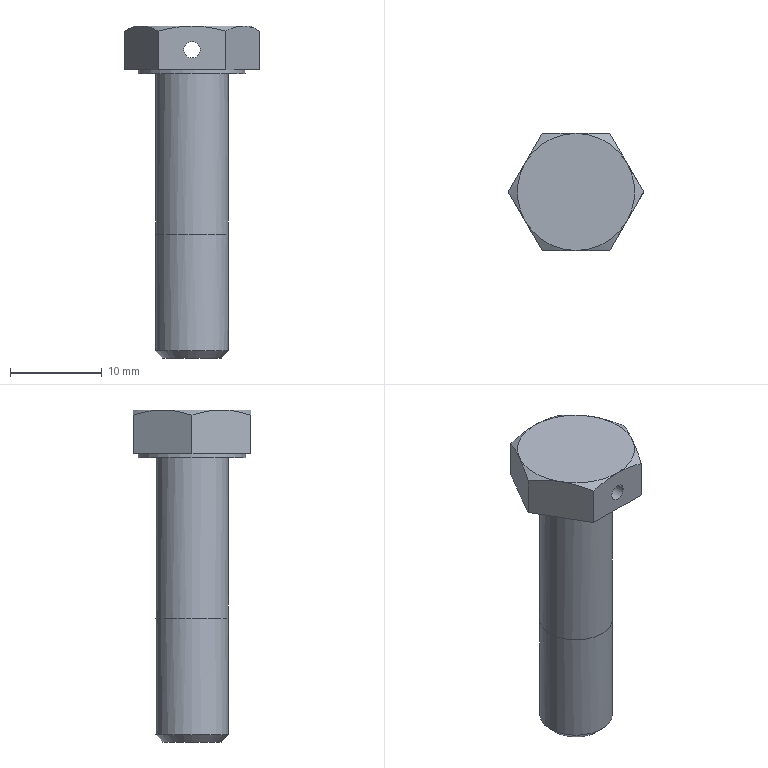Part | NX | features solid 2 | 1 solid | 21 faces | box 14.723 x 12.751 x 36.138 mm | volume 2207 mm3 | plane 10 | cone 7 | cylinder 4 | commonest cylinder face diameters 7.938 x2 1.778 x1 11.684 x1
STEP:
#1=CARTESIAN_POINT('',(-3.969,0.,-5.182));
#2=VERTEX_POINT('',#1);
#3=CARTESIAN_POINT('',(0.,0.,-5.182));
#4=DIRECTION('',(0.,0.,-1.));
#5=DIRECTION('',(-1.,0.,0.));
#6=AXIS2_PLACEMENT_3D('',#3,#4,#5);
#7=CIRCLE('',#6,3.969);
#8=EDGE_CURVE('',#2,#2,#7,.T.);
#9=ORIENTED_EDGE('',*,*,#8,.T.);
#10=EDGE_LOOP('',(#9));
#11=FACE_BOUND('',#10,.T.);
#12=CARTESIAN_POINT('',(-3.969,0.,-22.644));
#13=VERTEX_POINT('',#12);
#14=CARTESIAN_POINT('',(-3.11,3.11,-22.644));
#15=CARTESIAN_POINT('',(-4.398,0.,-22.644));
#16=CARTESIAN_POINT('',(-3.11,-3.11,-22.644));
#17=CARTESIAN_POINT('',(0.,-4.398,-22.644));
#18=CARTESIAN_POINT('',(3.11,-3.11,-22.644));
#19=CARTESIAN_POINT('',(4.398,0.,-22.644));
#20=CARTESIAN_POINT('',(3.11,3.11,-22.644));
#21=CARTESIAN_POINT('',(0.,4.398,-22.644));
#22=CARTESIAN_POINT('',(-3.11,3.11,-22.644));
#23=CARTESIAN_POINT('',(-4.398,0.,-22.644));
#24=CARTESIAN_POINT('',(-3.11,-3.11,-22.644));
#25=B_SPLINE_CURVE_WITH_KNOTS('',3,(#14,#15,#16,#17,#18,#19,#20,#21,#22,#23,#24),.UNSPECIFIED.,.T.,.F.,(1,1,1,1,1,1,1,1,1,1,1,1,1,1,1),(-0.375,-0.25,-0.125,0.,0.125,0.25,0.375,0.5,0.625,0.75,0.875,1.,1.125,1.25,1.375),.UNSPECIFIED.);
#26=EDGE_CURVE('',#13,#13,#25,.T.);
#27=ORIENTED_EDGE('',*,*,#26,.T.);
#28=EDGE_LOOP('',(#27));
#29=FACE_BOUND('',#28,.T.);
#30=CARTESIAN_POINT('',(0.,0.,0.));
#31=DIRECTION('',(0.,0.,-1.));
#32=DIRECTION('',(-1.,0.,0.));
#33=AXIS2_PLACEMENT_3D('',#30,#31,#32);
#34=CYLINDRICAL_SURFACE('',#33,3.969);
#35=ADVANCED_FACE('',(#11,#29),#34,.T.);
#36=CARTESIAN_POINT('',(-7.362,0.,-4.775));
#37=VERTEX_POINT('',#36);
#38=CARTESIAN_POINT('',(-3.681,6.375,-4.775));
#39=VERTEX_POINT('',#38);
#40=CARTESIAN_POINT('',(-4.061,5.717,-4.775));
#41=DIRECTION('',(0.5,0.866,0.));
#42=VECTOR('',#41,1000.);
#43=LINE('',#40,#42);
#44=EDGE_CURVE('',#37,#39,#43,.T.);
#45=ORIENTED_EDGE('',*,*,#44,.T.);
#46=CARTESIAN_POINT('',(3.681,6.375,-4.775));
#47=VERTEX_POINT('',#46);
#48=CARTESIAN_POINT('',(5.842,6.375,-4.775));
#49=DIRECTION('',(1.,0.,0.));
#50=VECTOR('',#49,1000.);
#51=LINE('',#48,#50);
#52=EDGE_CURVE('',#39,#47,#51,.T.);
#53=ORIENTED_EDGE('',*,*,#52,.T.);
#54=CARTESIAN_POINT('',(7.362,0.,-4.775));
#55=VERTEX_POINT('',#54);
#56=CARTESIAN_POINT('',(6.982,0.658,-4.775));
#57=DIRECTION('',(0.5,-0.866,0.));
#58=VECTOR('',#57,1000.);
#59=LINE('',#56,#58);
#60=EDGE_CURVE('',#47,#55,#59,.T.);
#61=ORIENTED_EDGE('',*,*,#60,.T.);
#62=CARTESIAN_POINT('',(3.681,-6.375,-4.775));
#63=VERTEX_POINT('',#62);
#64=CARTESIAN_POINT('',(6.982,-0.658,-4.775));
#65=DIRECTION('',(-0.5,-0.866,0.));
#66=VECTOR('',#65,1000.);
#67=LINE('',#64,#66);
#68=EDGE_CURVE('',#55,#63,#67,.T.);
#69=ORIENTED_EDGE('',*,*,#68,.T.);
#70=CARTESIAN_POINT('',(-3.681,-6.375,-4.775));
#71=VERTEX_POINT('',#70);
#72=CARTESIAN_POINT('',(5.842,-6.375,-4.775));
#73=DIRECTION('',(-1.,0.,0.));
#74=VECTOR('',#73,1000.);
#75=LINE('',#72,#74);
#76=EDGE_CURVE('',#63,#71,#75,.T.);
#77=ORIENTED_EDGE('',*,*,#76,.T.);
#78=CARTESIAN_POINT('',(-4.061,-5.717,-4.775));
#79=DIRECTION('',(-0.5,0.866,0.));
#80=VECTOR('',#79,1000.);
#81=LINE('',#78,#80);
#82=EDGE_CURVE('',#71,#37,#81,.T.);
#83=ORIENTED_EDGE('',*,*,#82,.T.);
#84=EDGE_LOOP('',(#45,#53,#61,#69,#77,#83));
#85=FACE_BOUND('',#84,.T.);
#86=CARTESIAN_POINT('',(-5.842,0.,-4.775));
#87=VERTEX_POINT('',#86);
#88=CARTESIAN_POINT('',(0.,0.,-4.775));
#89=DIRECTION('',(0.,0.,-1.));
#90=DIRECTION('',(-1.,0.,0.));
#91=AXIS2_PLACEMENT_3D('',#88,#89,#90);
#92=CIRCLE('',#91,5.842);
#93=EDGE_CURVE('',#87,#87,#92,.T.);
#94=ORIENTED_EDGE('',*,*,#93,.F.);
#95=EDGE_LOOP('',(#94));
#96=FACE_BOUND('',#95,.T.);
#97=CARTESIAN_POINT('',(5.842,0.,-4.775));
#98=DIRECTION('',(0.,0.,-1.));
#99=DIRECTION('',(-1.,0.,0.));
#100=AXIS2_PLACEMENT_3D('',#97,#98,#99);
#101=PLANE('',#100);
#102=ADVANCED_FACE('',(#85,#96),#101,.T.);
#103=CARTESIAN_POINT('',(-3.181,0.,-36.138));
#104=VERTEX_POINT('',#103);
#105=CARTESIAN_POINT('',(0.,0.,-36.138));
#106=DIRECTION('',(0.,0.,-1.));
#107=DIRECTION('',(-1.,0.,0.));
#108=AXIS2_PLACEMENT_3D('',#105,#106,#107);
#109=CIRCLE('',#108,3.181);
#110=EDGE_CURVE('',#104,#104,#109,.T.);
#111=ORIENTED_EDGE('',*,*,#110,.T.);
#112=EDGE_LOOP('',(#111));
#113=FACE_BOUND('',#112,.T.);
#114=CARTESIAN_POINT('',(0.,0.,-36.138));
#115=DIRECTION('',(0.,0.,-1.));
#116=DIRECTION('',(-1.,0.,0.));
#117=AXIS2_PLACEMENT_3D('',#114,#115,#116);
#118=PLANE('',#117);
#119=ADVANCED_FACE('',(#113),#118,.T.);
#120=CARTESIAN_POINT('',(-3.969,0.,-35.35));
#121=VERTEX_POINT('',#120);
#122=CARTESIAN_POINT('',(0.,0.,-35.35));
#123=DIRECTION('',(0.,0.,-1.));
#124=DIRECTION('',(-1.,0.,0.));
#125=AXIS2_PLACEMENT_3D('',#122,#123,#124);
#126=CIRCLE('',#125,3.969);
#127=EDGE_CURVE('',#121,#121,#126,.T.);
#128=ORIENTED_EDGE('',*,*,#127,.T.);
#129=EDGE_LOOP('',(#128));
#130=FACE_BOUND('',#129,.T.);
#131=ORIENTED_EDGE('',*,*,#110,.F.);
#132=EDGE_LOOP('',(#131));
#133=FACE_BOUND('',#132,.T.);
#134=CARTESIAN_POINT('',(0.,0.,-36.138));
#135=DIRECTION('',(0.,0.,1.));
#136=DIRECTION('',(1.,0.,0.));
#137=AXIS2_PLACEMENT_3D('',#134,#135,#136);
#138=CONICAL_SURFACE('',#137,3.181,0.7854);
#139=ADVANCED_FACE('',(#130,#133),#138,.T.);
#140=ORIENTED_EDGE('',*,*,#26,.F.);
#141=EDGE_LOOP('',(#140));
#142=FACE_BOUND('',#141,.T.);
#143=ORIENTED_EDGE('',*,*,#127,.F.);
#144=EDGE_LOOP('',(#143));
#145=FACE_BOUND('',#144,.T.);
#146=CARTESIAN_POINT('',(0.,0.,0.));
#147=DIRECTION('',(0.,0.,-1.));
#148=DIRECTION('',(-1.,0.,0.));
#149=AXIS2_PLACEMENT_3D('',#146,#147,#148);
#150=CYLINDRICAL_SURFACE('',#149,3.969);
#151=ADVANCED_FACE('',(#142,#145),#150,.T.);
#152=CARTESIAN_POINT('',(-5.842,0.,-5.182));
#153=VERTEX_POINT('',#152);
#154=CARTESIAN_POINT('',(0.,0.,-5.182));
#155=DIRECTION('',(0.,0.,-1.));
#156=DIRECTION('',(-1.,0.,0.));
#157=AXIS2_PLACEMENT_3D('',#154,#155,#156);
#158=CIRCLE('',#157,5.842);
#159=EDGE_CURVE('',#153,#153,#158,.T.);
#160=ORIENTED_EDGE('',*,*,#159,.T.);
#161=EDGE_LOOP('',(#160));
#162=FACE_BOUND('',#161,.T.);
#163=ORIENTED_EDGE('',*,*,#8,.F.);
#164=EDGE_LOOP('',(#163));
#165=FACE_BOUND('',#164,.T.);
#166=CARTESIAN_POINT('',(3.969,0.,-5.182));
#167=DIRECTION('',(0.,0.,-1.));
#168=DIRECTION('',(-1.,0.,0.));
#169=AXIS2_PLACEMENT_3D('',#166,#167,#168);
#170=PLANE('',#169);
#171=ADVANCED_FACE('',(#162,#165),#170,.T.);
#172=ORIENTED_EDGE('',*,*,#93,.T.);
#173=EDGE_LOOP('',(#172));
#174=FACE_BOUND('',#173,.T.);
#175=ORIENTED_EDGE('',*,*,#159,.F.);
#176=EDGE_LOOP('',(#175));
#177=FACE_BOUND('',#176,.T.);
#178=CARTESIAN_POINT('',(0.,0.,0.));
#179=DIRECTION('',(0.,0.,-1.));
#180=DIRECTION('',(-1.,0.,0.));
#181=AXIS2_PLACEMENT_3D('',#178,#179,#180);
#182=CYLINDRICAL_SURFACE('',#181,5.842);
#183=ADVANCED_FACE('',(#174,#177),#182,.T.);
#184=CARTESIAN_POINT('',(0.,6.375,-1.702));
#185=VERTEX_POINT('',#184);
#186=CARTESIAN_POINT('',(0.,6.375,-2.591));
#187=DIRECTION('',(0.,1.,0.));
#188=DIRECTION('',(0.,0.,1.));
#189=AXIS2_PLACEMENT_3D('',#186,#187,#188);
#190=CIRCLE('',#189,0.889);
#191=EDGE_CURVE('',#185,#185,#190,.T.);
#192=ORIENTED_EDGE('',*,*,#191,.F.);
#193=EDGE_LOOP('',(#192));
#194=FACE_BOUND('',#193,.T.);
#195=ORIENTED_EDGE('',*,*,#52,.F.);
#196=CARTESIAN_POINT('',(-3.681,6.375,-0.5694));
#197=VERTEX_POINT('',#196);
#198=CARTESIAN_POINT('',(-3.681,6.375,-39.752));
#199=DIRECTION('',(0.,0.,1.));
#200=VECTOR('',#199,1000.);
#201=LINE('',#198,#200);
#202=EDGE_CURVE('',#39,#197,#201,.T.);
#203=ORIENTED_EDGE('',*,*,#202,.T.);
#204=CARTESIAN_POINT('',(0.,6.375,0.));
#205=VERTEX_POINT('',#204);
#206=CARTESIAN_POINT('',(-3.681,6.375,-0.5694));
#207=CARTESIAN_POINT('',(-2.484,6.375,-0.2238));
#208=CARTESIAN_POINT('',(-1.244,6.375,0.));
#209=CARTESIAN_POINT('',(0.,6.375,0.));
#210=B_SPLINE_CURVE_WITH_KNOTS('',3,(#206,#207,#208,#209),.UNSPECIFIED.,.F.,.F.,(4,4),(0.006567,0.01029),.UNSPECIFIED.);
#211=EDGE_CURVE('',#205,#197,#210,.F.);
#212=ORIENTED_EDGE('',*,*,#211,.F.);
#213=CARTESIAN_POINT('',(3.681,6.375,-0.5694));
#214=VERTEX_POINT('',#213);
#215=CARTESIAN_POINT('',(0.,6.375,0.));
#216=CARTESIAN_POINT('',(1.245,6.375,0.));
#217=CARTESIAN_POINT('',(2.49,6.375,-0.2258));
#218=CARTESIAN_POINT('',(3.681,6.375,-0.5694));
#219=B_SPLINE_CURVE_WITH_KNOTS('',3,(#215,#216,#217,#218),.UNSPECIFIED.,.F.,.F.,(4,4),(0.01029,0.01402),.UNSPECIFIED.);
#220=EDGE_CURVE('',#214,#205,#219,.F.);
#221=ORIENTED_EDGE('',*,*,#220,.F.);
#222=CARTESIAN_POINT('',(3.681,6.375,-39.752));
#223=DIRECTION('',(0.,0.,1.));
#224=VECTOR('',#223,1000.);
#225=LINE('',#222,#224);
#226=EDGE_CURVE('',#47,#214,#225,.T.);
#227=ORIENTED_EDGE('',*,*,#226,.F.);
#228=EDGE_LOOP('',(#195,#203,#212,#221,#227));
#229=FACE_BOUND('',#228,.T.);
#230=CARTESIAN_POINT('',(3.681,6.375,-39.752));
#231=DIRECTION('',(0.,1.,0.));
#232=DIRECTION('',(0.,0.,1.));
#233=AXIS2_PLACEMENT_3D('',#230,#231,#232);
#234=PLANE('',#233);
#235=ADVANCED_FACE('',(#194,#229),#234,.T.);
#236=ORIENTED_EDGE('',*,*,#44,.F.);
#237=CARTESIAN_POINT('',(-7.362,0.,-0.5694));
#238=VERTEX_POINT('',#237);
#239=CARTESIAN_POINT('',(-7.362,0.,-39.752));
#240=DIRECTION('',(0.,0.,1.));
#241=VECTOR('',#240,1000.);
#242=LINE('',#239,#241);
#243=EDGE_CURVE('',#37,#238,#242,.T.);
#244=ORIENTED_EDGE('',*,*,#243,.T.);
#245=CARTESIAN_POINT('',(-5.521,3.188,0.));
#246=VERTEX_POINT('',#245);
#247=CARTESIAN_POINT('',(-5.521,3.188,0.));
#248=CARTESIAN_POINT('',(-6.146,2.106,0.));
#249=CARTESIAN_POINT('',(-6.761,1.04,-0.2227));
#250=CARTESIAN_POINT('',(-7.362,0.,-0.5694));
#251=B_SPLINE_CURVE_WITH_KNOTS('',3,(#247,#248,#249,#250),.UNSPECIFIED.,.F.,.F.,(4,4),(0.003725,0.007435),.UNSPECIFIED.);
#252=EDGE_CURVE('',#246,#238,#251,.T.);
#253=ORIENTED_EDGE('',*,*,#252,.F.);
#254=CARTESIAN_POINT('',(-3.681,6.375,-0.5694));
#255=CARTESIAN_POINT('',(-4.283,5.332,-0.2218));
#256=CARTESIAN_POINT('',(-4.894,4.274,0.));
#257=CARTESIAN_POINT('',(-5.521,3.188,0.));
#258=B_SPLINE_CURVE_WITH_KNOTS('',3,(#254,#255,#256,#257),.UNSPECIFIED.,.F.,.F.,(4,4),(0.000000238,0.003725),.UNSPECIFIED.);
#259=EDGE_CURVE('',#197,#246,#258,.T.);
#260=ORIENTED_EDGE('',*,*,#259,.F.);
#261=ORIENTED_EDGE('',*,*,#202,.F.);
#262=EDGE_LOOP('',(#236,#244,#253,#260,#261));
#263=FACE_BOUND('',#262,.T.);
#264=CARTESIAN_POINT('',(-3.681,6.375,-39.752));
#265=DIRECTION('',(-0.866,0.5,0.));
#266=DIRECTION('',(-0.5,-0.866,0.));
#267=AXIS2_PLACEMENT_3D('',#264,#265,#266);
#268=PLANE('',#267);
#269=ADVANCED_FACE('',(#263),#268,.T.);
#270=ORIENTED_EDGE('',*,*,#82,.F.);
#271=CARTESIAN_POINT('',(-3.681,-6.375,-0.5694));
#272=VERTEX_POINT('',#271);
#273=CARTESIAN_POINT('',(-3.681,-6.375,-39.752));
#274=DIRECTION('',(0.,0.,1.));
#275=VECTOR('',#274,1000.);
#276=LINE('',#273,#275);
#277=EDGE_CURVE('',#71,#272,#276,.T.);
#278=ORIENTED_EDGE('',*,*,#277,.T.);
#279=CARTESIAN_POINT('',(-5.521,-3.188,0.));
#280=VERTEX_POINT('',#279);
#281=CARTESIAN_POINT('',(-5.521,-3.188,0.));
#282=CARTESIAN_POINT('',(-4.896,-4.27,0.));
#283=CARTESIAN_POINT('',(-4.281,-5.335,-0.2227));
#284=CARTESIAN_POINT('',(-3.681,-6.375,-0.5694));
#285=B_SPLINE_CURVE_WITH_KNOTS('',3,(#281,#282,#283,#284),.UNSPECIFIED.,.F.,.F.,(4,4),(0.003725,0.007435),.UNSPECIFIED.);
#286=EDGE_CURVE('',#280,#272,#285,.T.);
#287=ORIENTED_EDGE('',*,*,#286,.F.);
#288=CARTESIAN_POINT('',(-7.362,0.,-0.5694));
#289=CARTESIAN_POINT('',(-6.76,-1.043,-0.2218));
#290=CARTESIAN_POINT('',(-6.148,-2.102,0.));
#291=CARTESIAN_POINT('',(-5.521,-3.188,0.));
#292=B_SPLINE_CURVE_WITH_KNOTS('',3,(#288,#289,#290,#291),.UNSPECIFIED.,.F.,.F.,(4,4),(0.000000238,0.003725),.UNSPECIFIED.);
#293=EDGE_CURVE('',#238,#280,#292,.T.);
#294=ORIENTED_EDGE('',*,*,#293,.F.);
#295=ORIENTED_EDGE('',*,*,#243,.F.);
#296=EDGE_LOOP('',(#270,#278,#287,#294,#295));
#297=FACE_BOUND('',#296,.T.);
#298=CARTESIAN_POINT('',(-7.362,0.,-39.752));
#299=DIRECTION('',(-0.866,-0.5,0.));
#300=DIRECTION('',(0.5,-0.866,0.));
#301=AXIS2_PLACEMENT_3D('',#298,#299,#300);
#302=PLANE('',#301);
#303=ADVANCED_FACE('',(#297),#302,.T.);
#304=CARTESIAN_POINT('',(0.,-6.375,-3.48));
#305=VERTEX_POINT('',#304);
#306=CARTESIAN_POINT('',(0.,-6.375,-2.591));
#307=DIRECTION('',(0.,-1.,0.));
#308=DIRECTION('',(0.,0.,-1.));
#309=AXIS2_PLACEMENT_3D('',#306,#307,#308);
#310=CIRCLE('',#309,0.889);
#311=EDGE_CURVE('',#305,#305,#310,.T.);
#312=ORIENTED_EDGE('',*,*,#311,.F.);
#313=EDGE_LOOP('',(#312));
#314=FACE_BOUND('',#313,.T.);
#315=ORIENTED_EDGE('',*,*,#76,.F.);
#316=CARTESIAN_POINT('',(3.681,-6.375,-0.5694));
#317=VERTEX_POINT('',#316);
#318=CARTESIAN_POINT('',(3.681,-6.375,-39.752));
#319=DIRECTION('',(0.,0.,1.));
#320=VECTOR('',#319,1000.);
#321=LINE('',#318,#320);
#322=EDGE_CURVE('',#63,#317,#321,.T.);
#323=ORIENTED_EDGE('',*,*,#322,.T.);
#324=CARTESIAN_POINT('',(0.,-6.375,0.));
#325=VERTEX_POINT('',#324);
#326=CARTESIAN_POINT('',(0.,-6.375,0.));
#327=CARTESIAN_POINT('',(1.245,-6.375,0.));
#328=CARTESIAN_POINT('',(2.49,-6.375,-0.2258));
#329=CARTESIAN_POINT('',(3.681,-6.375,-0.5694));
#330=B_SPLINE_CURVE_WITH_KNOTS('',3,(#326,#327,#328,#329),.UNSPECIFIED.,.F.,.F.,(4,4),(0.01029,0.01402),.UNSPECIFIED.);
#331=EDGE_CURVE('',#325,#317,#330,.T.);
#332=ORIENTED_EDGE('',*,*,#331,.F.);
#333=CARTESIAN_POINT('',(-3.681,-6.375,-0.5694));
#334=CARTESIAN_POINT('',(-2.484,-6.375,-0.2238));
#335=CARTESIAN_POINT('',(-1.244,-6.375,0.));
#336=CARTESIAN_POINT('',(0.,-6.375,0.));
#337=B_SPLINE_CURVE_WITH_KNOTS('',3,(#333,#334,#335,#336),.UNSPECIFIED.,.F.,.F.,(4,4),(0.006567,0.01029),.UNSPECIFIED.);
#338=EDGE_CURVE('',#272,#325,#337,.T.);
#339=ORIENTED_EDGE('',*,*,#338,.F.);
#340=ORIENTED_EDGE('',*,*,#277,.F.);
#341=EDGE_LOOP('',(#315,#323,#332,#339,#340));
#342=FACE_BOUND('',#341,.T.);
#343=CARTESIAN_POINT('',(-3.681,-6.375,-39.752));
#344=DIRECTION('',(0.,-1.,0.));
#345=DIRECTION('',(0.,0.,-1.));
#346=AXIS2_PLACEMENT_3D('',#343,#344,#345);
#347=PLANE('',#346);
#348=ADVANCED_FACE('',(#314,#342),#347,.T.);
#349=ORIENTED_EDGE('',*,*,#68,.F.);
#350=CARTESIAN_POINT('',(7.362,0.,-0.5694));
#351=VERTEX_POINT('',#350);
#352=CARTESIAN_POINT('',(7.362,0.,-39.752));
#353=DIRECTION('',(0.,0.,1.));
#354=VECTOR('',#353,1000.);
#355=LINE('',#352,#354);
#356=EDGE_CURVE('',#55,#351,#355,.T.);
#357=ORIENTED_EDGE('',*,*,#356,.T.);
#358=CARTESIAN_POINT('',(5.521,-3.188,0.));
#359=VERTEX_POINT('',#358);
#360=CARTESIAN_POINT('',(5.521,-3.188,0.));
#361=CARTESIAN_POINT('',(6.146,-2.106,0.));
#362=CARTESIAN_POINT('',(6.761,-1.04,-0.2227));
#363=CARTESIAN_POINT('',(7.362,0.,-0.5694));
#364=B_SPLINE_CURVE_WITH_KNOTS('',3,(#360,#361,#362,#363),.UNSPECIFIED.,.F.,.F.,(4,4),(0.003725,0.007435),.UNSPECIFIED.);
#365=EDGE_CURVE('',#359,#351,#364,.T.);
#366=ORIENTED_EDGE('',*,*,#365,.F.);
#367=CARTESIAN_POINT('',(3.681,-6.375,-0.5694));
#368=CARTESIAN_POINT('',(4.283,-5.332,-0.2218));
#369=CARTESIAN_POINT('',(4.894,-4.274,0.));
#370=CARTESIAN_POINT('',(5.521,-3.188,0.));
#371=B_SPLINE_CURVE_WITH_KNOTS('',3,(#367,#368,#369,#370),.UNSPECIFIED.,.F.,.F.,(4,4),(0.000000238,0.003725),.UNSPECIFIED.);
#372=EDGE_CURVE('',#317,#359,#371,.T.);
#373=ORIENTED_EDGE('',*,*,#372,.F.);
#374=ORIENTED_EDGE('',*,*,#322,.F.);
#375=EDGE_LOOP('',(#349,#357,#366,#373,#374));
#376=FACE_BOUND('',#375,.T.);
#377=CARTESIAN_POINT('',(3.681,-6.375,-39.752));
#378=DIRECTION('',(0.866,-0.5,0.));
#379=DIRECTION('',(0.5,0.866,0.));
#380=AXIS2_PLACEMENT_3D('',#377,#378,#379);
#381=PLANE('',#380);
#382=ADVANCED_FACE('',(#376),#381,.T.);
#383=ORIENTED_EDGE('',*,*,#60,.F.);
#384=ORIENTED_EDGE('',*,*,#226,.T.);
#385=CARTESIAN_POINT('',(5.521,3.188,0.));
#386=VERTEX_POINT('',#385);
#387=CARTESIAN_POINT('',(5.521,3.188,0.));
#388=CARTESIAN_POINT('',(4.896,4.27,0.));
#389=CARTESIAN_POINT('',(4.281,5.335,-0.2227));
#390=CARTESIAN_POINT('',(3.681,6.375,-0.5694));
#391=B_SPLINE_CURVE_WITH_KNOTS('',3,(#387,#388,#389,#390),.UNSPECIFIED.,.F.,.F.,(4,4),(0.003725,0.007435),.UNSPECIFIED.);
#392=EDGE_CURVE('',#386,#214,#391,.T.);
#393=ORIENTED_EDGE('',*,*,#392,.F.);
#394=CARTESIAN_POINT('',(7.362,0.,-0.5694));
#395=CARTESIAN_POINT('',(6.76,1.043,-0.2218));
#396=CARTESIAN_POINT('',(6.148,2.102,0.));
#397=CARTESIAN_POINT('',(5.521,3.188,0.));
#398=B_SPLINE_CURVE_WITH_KNOTS('',3,(#394,#395,#396,#397),.UNSPECIFIED.,.F.,.F.,(4,4),(0.000000238,0.003725),.UNSPECIFIED.);
#399=EDGE_CURVE('',#351,#386,#398,.T.);
#400=ORIENTED_EDGE('',*,*,#399,.F.);
#401=ORIENTED_EDGE('',*,*,#356,.F.);
#402=EDGE_LOOP('',(#383,#384,#393,#400,#401));
#403=FACE_BOUND('',#402,.T.);
#404=CARTESIAN_POINT('',(7.362,0.,-39.752));
#405=DIRECTION('',(0.866,0.5,0.));
#406=DIRECTION('',(-0.5,0.866,0.));
#407=AXIS2_PLACEMENT_3D('',#404,#405,#406);
#408=PLANE('',#407);
#409=ADVANCED_FACE('',(#403),#408,.T.);
#410=CARTESIAN_POINT('',(0.,0.,0.));
#411=DIRECTION('',(0.,0.,-1.));
#412=DIRECTION('',(-1.,0.,0.));
#413=AXIS2_PLACEMENT_3D('',#410,#411,#412);
#414=CIRCLE('',#413,6.375);
#415=EDGE_CURVE('',#386,#359,#414,.T.);
#416=ORIENTED_EDGE('',*,*,#415,.T.);
#417=ORIENTED_EDGE('',*,*,#365,.T.);
#418=ORIENTED_EDGE('',*,*,#399,.T.);
#419=EDGE_LOOP('',(#416,#417,#418));
#420=FACE_BOUND('',#419,.T.);
#421=CARTESIAN_POINT('',(0.,0.,-0.5719));
#422=DIRECTION('',(0.,0.,-1.));
#423=DIRECTION('',(-1.,0.,0.));
#424=AXIS2_PLACEMENT_3D('',#421,#422,#423);
#425=CONICAL_SURFACE('',#424,7.366,1.047);
#426=ADVANCED_FACE('',(#420),#425,.T.);
#427=CARTESIAN_POINT('',(0.,0.,0.));
#428=DIRECTION('',(0.,0.,-1.));
#429=DIRECTION('',(-1.,0.,0.));
#430=AXIS2_PLACEMENT_3D('',#427,#428,#429);
#431=CIRCLE('',#430,6.375);
#432=EDGE_CURVE('',#359,#325,#431,.T.);
#433=ORIENTED_EDGE('',*,*,#432,.T.);
#434=ORIENTED_EDGE('',*,*,#331,.T.);
#435=ORIENTED_EDGE('',*,*,#372,.T.);
#436=EDGE_LOOP('',(#433,#434,#435));
#437=FACE_BOUND('',#436,.T.);
#438=CARTESIAN_POINT('',(0.,0.,-0.5719));
#439=DIRECTION('',(0.,0.,-1.));
#440=DIRECTION('',(-1.,0.,0.));
#441=AXIS2_PLACEMENT_3D('',#438,#439,#440);
#442=CONICAL_SURFACE('',#441,7.366,1.047);
#443=ADVANCED_FACE('',(#437),#442,.T.);
#444=CARTESIAN_POINT('',(0.,0.,0.));
#445=DIRECTION('',(0.,0.,-1.));
#446=DIRECTION('',(-1.,0.,0.));
#447=AXIS2_PLACEMENT_3D('',#444,#445,#446);
#448=CIRCLE('',#447,6.375);
#449=EDGE_CURVE('',#325,#280,#448,.T.);
#450=ORIENTED_EDGE('',*,*,#449,.T.);
#451=ORIENTED_EDGE('',*,*,#286,.T.);
#452=ORIENTED_EDGE('',*,*,#338,.T.);
#453=EDGE_LOOP('',(#450,#451,#452));
#454=FACE_BOUND('',#453,.T.);
#455=CARTESIAN_POINT('',(0.,0.,-0.5719));
#456=DIRECTION('',(0.,0.,-1.));
#457=DIRECTION('',(-1.,0.,0.));
#458=AXIS2_PLACEMENT_3D('',#455,#456,#457);
#459=CONICAL_SURFACE('',#458,7.366,1.047);
#460=ADVANCED_FACE('',(#454),#459,.T.);
#461=CARTESIAN_POINT('',(0.,0.,0.));
#462=DIRECTION('',(0.,0.,-1.));
#463=DIRECTION('',(-1.,0.,0.));
#464=AXIS2_PLACEMENT_3D('',#461,#462,#463);
#465=CIRCLE('',#464,6.375);
#466=EDGE_CURVE('',#280,#246,#465,.T.);
#467=ORIENTED_EDGE('',*,*,#466,.T.);
#468=ORIENTED_EDGE('',*,*,#252,.T.);
#469=ORIENTED_EDGE('',*,*,#293,.T.);
#470=EDGE_LOOP('',(#467,#468,#469));
#471=FACE_BOUND('',#470,.T.);
#472=CARTESIAN_POINT('',(0.,0.,-0.5719));
#473=DIRECTION('',(0.,0.,-1.));
#474=DIRECTION('',(-1.,0.,0.));
#475=AXIS2_PLACEMENT_3D('',#472,#473,#474);
#476=CONICAL_SURFACE('',#475,7.366,1.047);
#477=ADVANCED_FACE('',(#471),#476,.T.);
#478=CARTESIAN_POINT('',(0.,0.,0.));
#479=DIRECTION('',(0.,0.,-1.));
#480=DIRECTION('',(-1.,0.,0.));
#481=AXIS2_PLACEMENT_3D('',#478,#479,#480);
#482=CIRCLE('',#481,6.375);
#483=EDGE_CURVE('',#246,#205,#482,.T.);
#484=ORIENTED_EDGE('',*,*,#483,.T.);
#485=ORIENTED_EDGE('',*,*,#211,.T.);
#486=ORIENTED_EDGE('',*,*,#259,.T.);
#487=EDGE_LOOP('',(#484,#485,#486));
#488=FACE_BOUND('',#487,.T.);
#489=CARTESIAN_POINT('',(0.,0.,-0.5719));
#490=DIRECTION('',(0.,0.,-1.));
#491=DIRECTION('',(-1.,0.,0.));
#492=AXIS2_PLACEMENT_3D('',#489,#490,#491);
#493=CONICAL_SURFACE('',#492,7.366,1.047);
#494=ADVANCED_FACE('',(#488),#493,.T.);
#495=ORIENTED_EDGE('',*,*,#483,.F.);
#496=ORIENTED_EDGE('',*,*,#466,.F.);
#497=ORIENTED_EDGE('',*,*,#449,.F.);
#498=ORIENTED_EDGE('',*,*,#432,.F.);
#499=ORIENTED_EDGE('',*,*,#415,.F.);
#500=CARTESIAN_POINT('',(0.,0.,0.));
#501=DIRECTION('',(0.,0.,-1.));
#502=DIRECTION('',(-1.,0.,0.));
#503=AXIS2_PLACEMENT_3D('',#500,#501,#502);
#504=CIRCLE('',#503,6.375);
#505=EDGE_CURVE('',#205,#386,#504,.T.);
#506=ORIENTED_EDGE('',*,*,#505,.F.);
#507=EDGE_LOOP('',(#495,#496,#497,#498,#499,#506));
#508=FACE_BOUND('',#507,.T.);
#509=CARTESIAN_POINT('',(6.375,0.,0.));
#510=DIRECTION('',(0.,0.,1.));
#511=DIRECTION('',(1.,0.,0.));
#512=AXIS2_PLACEMENT_3D('',#509,#510,#511);
#513=PLANE('',#512);
#514=ADVANCED_FACE('',(#508),#513,.T.);
#515=ORIENTED_EDGE('',*,*,#392,.T.);
#516=ORIENTED_EDGE('',*,*,#220,.T.);
#517=ORIENTED_EDGE('',*,*,#505,.T.);
#518=EDGE_LOOP('',(#515,#516,#517));
#519=FACE_BOUND('',#518,.T.);
#520=CARTESIAN_POINT('',(0.,0.,-0.5719));
#521=DIRECTION('',(0.,0.,-1.));
#522=DIRECTION('',(-1.,0.,0.));
#523=AXIS2_PLACEMENT_3D('',#520,#521,#522);
#524=CONICAL_SURFACE('',#523,7.366,1.047);
#525=ADVANCED_FACE('',(#519),#524,.T.);
#526=ORIENTED_EDGE('',*,*,#191,.T.);
#527=EDGE_LOOP('',(#526));
#528=FACE_BOUND('',#527,.T.);
#529=ORIENTED_EDGE('',*,*,#311,.T.);
#530=EDGE_LOOP('',(#529));
#531=FACE_BOUND('',#530,.T.);
#532=CARTESIAN_POINT('',(0.,7.013,-2.591));
#533=DIRECTION('',(0.,-1.,0.));
#534=DIRECTION('',(0.,0.,-1.));
#535=AXIS2_PLACEMENT_3D('',#532,#533,#534);
#536=CYLINDRICAL_SURFACE('',#535,0.889);
#537=ADVANCED_FACE('',(#528,#531),#536,.F.);
#538=CLOSED_SHELL('',(#35,#102,#119,#139,#151,#171,#183,#235,#269,#303,#348,#382,#409,#426,#443,#460,#477,#494,#514,#525,#537));
#539=MANIFOLD_SOLID_BREP('',#538);
#540=(LENGTH_UNIT()NAMED_UNIT(*)SI_UNIT(.MILLI.,.METRE.));
#541=UNCERTAINTY_MEASURE_WITH_UNIT(LENGTH_MEASURE(0.0508),#540,'','');
#542=(NAMED_UNIT(*)PLANE_ANGLE_UNIT()SI_UNIT($,.RADIAN.));
#543=(NAMED_UNIT(*)SI_UNIT($,.STERADIAN.)SOLID_ANGLE_UNIT());
#544=(GEOMETRIC_REPRESENTATION_CONTEXT(3)GLOBAL_UNCERTAINTY_ASSIGNED_CONTEXT((#541))GLOBAL_UNIT_ASSIGNED_CONTEXT((#540,#542,#543))REPRESENTATION_CONTEXT('',''));
#545=ADVANCED_BREP_SHAPE_REPRESENTATION('',(#539),#544);